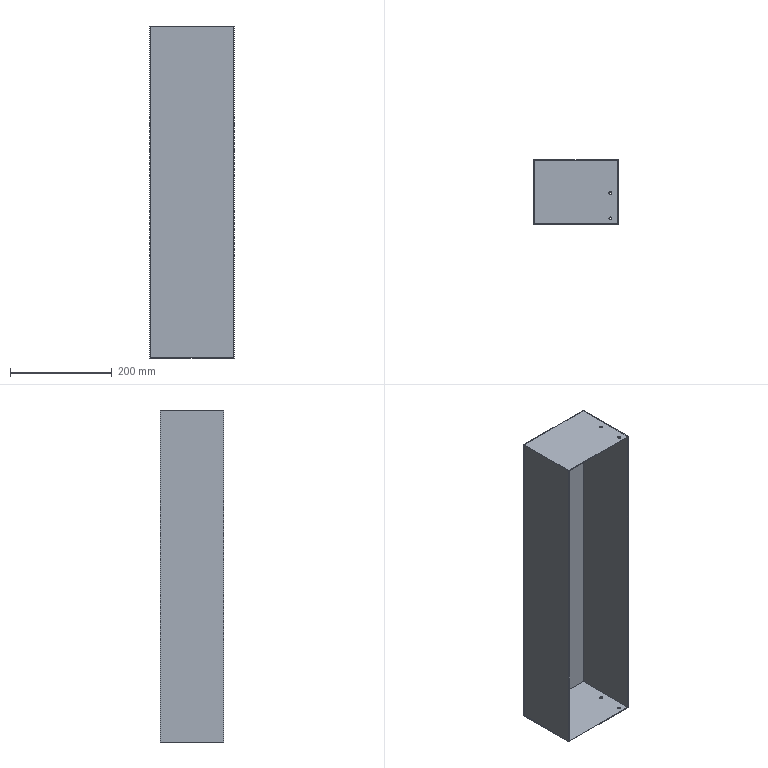Part | STEP file | 1 solid | 19 faces | box 165 x 125 x 652 mm | volume 309587 mm3 | plane 11 | cylinder 8 | commonest cylinder face diameters 6 x8
STEP:
#1=CARTESIAN_POINT('',(0.,0.,0.));
#2=DIRECTION('',(0.,0.,1.));
#3=DIRECTION('',(1.,0.,0.));
#4=AXIS2_PLACEMENT_3D('',#1,#2,#3);
#5=CARTESIAN_POINT('',(-18.,745.,652.));
#6=VERTEX_POINT('',#5);
#7=CARTESIAN_POINT('',(-18.,745.,651.));
#8=VERTEX_POINT('',#7);
#9=CARTESIAN_POINT('',(-18.,745.,652.));
#10=DIRECTION('',(0.,0.,-1.));
#11=VECTOR('',#10,1.);
#12=LINE('',#9,#11);
#13=CARTESIAN_POINT('',(-15.,745.,652.));
#14=DIRECTION('',(0.,0.,-1.));
#15=DIRECTION('',(-1.,0.,0.));
#16=AXIS2_PLACEMENT_3D('',#13,#14,#15);
#17=CYLINDRICAL_SURFACE('',#16,3.);
#18=CARTESIAN_POINT('',(6.283,0.));
#19=DIRECTION('',(0.,1.));
#20=VECTOR('',#19,1.);
#21=LINE('',#18,#20);
#22=(GEOMETRIC_REPRESENTATION_CONTEXT(2)PARAMETRIC_REPRESENTATION_CONTEXT()REPRESENTATION_CONTEXT('',''));
#23=DEFINITIONAL_REPRESENTATION('',(#21),#22);
#24=PCURVE('',#17,#23);
#25=CARTESIAN_POINT('',(-15.,745.,652.));
#26=DIRECTION('',(0.,0.,-1.));
#27=DIRECTION('',(-1.,0.,0.));
#28=AXIS2_PLACEMENT_3D('',#25,#26,#27);
#29=CYLINDRICAL_SURFACE('',#28,3.);
#30=CARTESIAN_POINT('',(0.,0.));
#31=DIRECTION('',(0.,1.));
#32=VECTOR('',#31,1.);
#33=LINE('',#30,#32);
#34=(GEOMETRIC_REPRESENTATION_CONTEXT(2)PARAMETRIC_REPRESENTATION_CONTEXT()REPRESENTATION_CONTEXT('',''));
#35=DEFINITIONAL_REPRESENTATION('',(#33),#34);
#36=PCURVE('',#29,#35);
#37=SURFACE_CURVE('',#12,(#24,#36),.PCURVE_S1.);
#38=EDGE_CURVE('',#6,#8,#37,.T.);
#39=ORIENTED_EDGE('',*,*,#38,.T.);
#40=CARTESIAN_POINT('',(-12.,745.,651.));
#41=VERTEX_POINT('',#40);
#42=CARTESIAN_POINT('',(-15.,745.,651.));
#43=DIRECTION('',(0.,0.,1.));
#44=DIRECTION('',(1.,0.,0.));
#45=AXIS2_PLACEMENT_3D('',#42,#43,#44);
#46=CIRCLE('',#45,3.);
#47=CARTESIAN_POINT('',(9.425,1.));
#48=DIRECTION('',(-1.,0.));
#49=VECTOR('',#48,1.);
#50=LINE('',#47,#49);
#51=(GEOMETRIC_REPRESENTATION_CONTEXT(2)PARAMETRIC_REPRESENTATION_CONTEXT()REPRESENTATION_CONTEXT('',''));
#52=DEFINITIONAL_REPRESENTATION('',(#50),#51);
#53=PCURVE('',#17,#52);
#54=CARTESIAN_POINT('',(0.,0.,651.));
#55=DIRECTION('',(0.,0.,1.));
#56=DIRECTION('',(1.,0.,0.));
#57=AXIS2_PLACEMENT_3D('',#54,#55,#56);
#58=PLANE('',#57);
#59=CARTESIAN_POINT('',(-15.,745.));
#60=DIRECTION('',(1.,0.));
#61=AXIS2_PLACEMENT_2D('',#59,#60);
#62=CIRCLE('',#61,3.);
#63=(GEOMETRIC_REPRESENTATION_CONTEXT(2)PARAMETRIC_REPRESENTATION_CONTEXT()REPRESENTATION_CONTEXT('',''));
#64=DEFINITIONAL_REPRESENTATION('',(#62),#63);
#65=PCURVE('',#58,#64);
#66=SURFACE_CURVE('',#46,(#53,#65),.PCURVE_S1.);
#67=EDGE_CURVE('',#8,#41,#66,.T.);
#68=ORIENTED_EDGE('',*,*,#67,.T.);
#69=CARTESIAN_POINT('',(-12.,745.,652.));
#70=VERTEX_POINT('',#69);
#71=CARTESIAN_POINT('',(-12.,745.,652.));
#72=DIRECTION('',(0.,0.,-1.));
#73=VECTOR('',#72,1.);
#74=LINE('',#71,#73);
#75=CARTESIAN_POINT('',(3.142,0.));
#76=DIRECTION('',(0.,1.));
#77=VECTOR('',#76,1.);
#78=LINE('',#75,#77);
#79=(GEOMETRIC_REPRESENTATION_CONTEXT(2)PARAMETRIC_REPRESENTATION_CONTEXT()REPRESENTATION_CONTEXT('',''));
#80=DEFINITIONAL_REPRESENTATION('',(#78),#79);
#81=PCURVE('',#17,#80);
#82=CARTESIAN_POINT('',(3.142,0.));
#83=DIRECTION('',(0.,1.));
#84=VECTOR('',#83,1.);
#85=LINE('',#82,#84);
#86=(GEOMETRIC_REPRESENTATION_CONTEXT(2)PARAMETRIC_REPRESENTATION_CONTEXT()REPRESENTATION_CONTEXT('',''));
#87=DEFINITIONAL_REPRESENTATION('',(#85),#86);
#88=PCURVE('',#29,#87);
#89=SURFACE_CURVE('',#74,(#81,#88),.PCURVE_S1.);
#90=EDGE_CURVE('',#70,#41,#89,.T.);
#91=ORIENTED_EDGE('',*,*,#90,.F.);
#92=CARTESIAN_POINT('',(-15.,745.,652.));
#93=DIRECTION('',(0.,0.,-1.));
#94=DIRECTION('',(-1.,0.,0.));
#95=AXIS2_PLACEMENT_3D('',#92,#93,#94);
#96=CIRCLE('',#95,3.);
#97=CARTESIAN_POINT('',(0.,0.));
#98=DIRECTION('',(1.,0.));
#99=VECTOR('',#98,1.);
#100=LINE('',#97,#99);
#101=(GEOMETRIC_REPRESENTATION_CONTEXT(2)PARAMETRIC_REPRESENTATION_CONTEXT()REPRESENTATION_CONTEXT('',''));
#102=DEFINITIONAL_REPRESENTATION('',(#100),#101);
#103=PCURVE('',#17,#102);
#104=CARTESIAN_POINT('',(0.,0.,652.));
#105=DIRECTION('',(0.,0.,1.));
#106=DIRECTION('',(1.,0.,0.));
#107=AXIS2_PLACEMENT_3D('',#104,#105,#106);
#108=PLANE('',#107);
#109=CARTESIAN_POINT('',(-18.,745.));
#110=CARTESIAN_POINT('',(-18.,750.196));
#111=CARTESIAN_POINT('',(-13.5,747.598));
#112=CARTESIAN_POINT('',(-9.,745.));
#113=CARTESIAN_POINT('',(-13.5,742.402));
#114=CARTESIAN_POINT('',(-18.,739.804));
#115=CARTESIAN_POINT('',(-18.,745.));
#116=(BOUNDED_CURVE()B_SPLINE_CURVE(2,(#109,#110,#111,#112,#113,#114,#115),.UNSPECIFIED.,.T.,.F.)B_SPLINE_CURVE_WITH_KNOTS((1,2,2,2,2,1),(-2.094,0.,2.094,4.189,6.283,8.378),.UNSPECIFIED.)CURVE()GEOMETRIC_REPRESENTATION_ITEM()RATIONAL_B_SPLINE_CURVE((1.,0.5,1.,0.5,1.,0.5,1.))REPRESENTATION_ITEM(''));
#117=(GEOMETRIC_REPRESENTATION_CONTEXT(2)PARAMETRIC_REPRESENTATION_CONTEXT()REPRESENTATION_CONTEXT('',''));
#118=DEFINITIONAL_REPRESENTATION('',(#116),#117);
#119=PCURVE('',#108,#118);
#120=SURFACE_CURVE('',#96,(#103,#119),.PCURVE_S1.);
#121=EDGE_CURVE('',#70,#6,#120,.T.);
#122=ORIENTED_EDGE('',*,*,#121,.T.);
#123=EDGE_LOOP('',(#39,#68,#91,#122));
#124=FACE_BOUND('',#123,.F.);
#125=ADVANCED_FACE('',(#124),#17,.F.);
#126=CARTESIAN_POINT('',(-18.,745.,1.));
#127=VERTEX_POINT('',#126);
#128=CARTESIAN_POINT('',(-18.,745.,0.));
#129=VERTEX_POINT('',#128);
#130=CARTESIAN_POINT('',(-18.,745.,652.));
#131=DIRECTION('',(0.,0.,-1.));
#132=VECTOR('',#131,1.);
#133=LINE('',#130,#132);
#134=CARTESIAN_POINT('',(-15.,745.,652.));
#135=DIRECTION('',(0.,0.,-1.));
#136=DIRECTION('',(-1.,0.,0.));
#137=AXIS2_PLACEMENT_3D('',#134,#135,#136);
#138=CYLINDRICAL_SURFACE('',#137,3.);
#139=CARTESIAN_POINT('',(6.283,0.));
#140=DIRECTION('',(0.,1.));
#141=VECTOR('',#140,1.);
#142=LINE('',#139,#141);
#143=(GEOMETRIC_REPRESENTATION_CONTEXT(2)PARAMETRIC_REPRESENTATION_CONTEXT()REPRESENTATION_CONTEXT('',''));
#144=DEFINITIONAL_REPRESENTATION('',(#142),#143);
#145=PCURVE('',#138,#144);
#146=CARTESIAN_POINT('',(-15.,745.,652.));
#147=DIRECTION('',(0.,0.,-1.));
#148=DIRECTION('',(-1.,0.,0.));
#149=AXIS2_PLACEMENT_3D('',#146,#147,#148);
#150=CYLINDRICAL_SURFACE('',#149,3.);
#151=CARTESIAN_POINT('',(0.,0.));
#152=DIRECTION('',(0.,1.));
#153=VECTOR('',#152,1.);
#154=LINE('',#151,#153);
#155=(GEOMETRIC_REPRESENTATION_CONTEXT(2)PARAMETRIC_REPRESENTATION_CONTEXT()REPRESENTATION_CONTEXT('',''));
#156=DEFINITIONAL_REPRESENTATION('',(#154),#155);
#157=PCURVE('',#150,#156);
#158=SURFACE_CURVE('',#133,(#145,#157),.PCURVE_S1.);
#159=EDGE_CURVE('',#127,#129,#158,.T.);
#160=ORIENTED_EDGE('',*,*,#159,.T.);
#161=CARTESIAN_POINT('',(-12.,745.,0.));
#162=VERTEX_POINT('',#161);
#163=CARTESIAN_POINT('',(-15.,745.,0.));
#164=DIRECTION('',(0.,0.,-1.));
#165=DIRECTION('',(-1.,0.,0.));
#166=AXIS2_PLACEMENT_3D('',#163,#164,#165);
#167=CIRCLE('',#166,3.);
#168=CARTESIAN_POINT('',(0.,652.));
#169=DIRECTION('',(1.,0.));
#170=VECTOR('',#169,1.);
#171=LINE('',#168,#170);
#172=(GEOMETRIC_REPRESENTATION_CONTEXT(2)PARAMETRIC_REPRESENTATION_CONTEXT()REPRESENTATION_CONTEXT('',''));
#173=DEFINITIONAL_REPRESENTATION('',(#171),#172);
#174=PCURVE('',#138,#173);
#175=CARTESIAN_POINT('',(0.,0.,0.));
#176=DIRECTION('',(0.,0.,1.));
#177=DIRECTION('',(1.,0.,0.));
#178=AXIS2_PLACEMENT_3D('',#175,#176,#177);
#179=PLANE('',#178);
#180=CARTESIAN_POINT('',(-18.,745.));
#181=CARTESIAN_POINT('',(-18.,750.196));
#182=CARTESIAN_POINT('',(-13.5,747.598));
#183=CARTESIAN_POINT('',(-9.,745.));
#184=CARTESIAN_POINT('',(-13.5,742.402));
#185=CARTESIAN_POINT('',(-18.,739.804));
#186=CARTESIAN_POINT('',(-18.,745.));
#187=(BOUNDED_CURVE()B_SPLINE_CURVE(2,(#180,#181,#182,#183,#184,#185,#186),.UNSPECIFIED.,.T.,.F.)B_SPLINE_CURVE_WITH_KNOTS((1,2,2,2,2,1),(-2.094,0.,2.094,4.189,6.283,8.378),.UNSPECIFIED.)CURVE()GEOMETRIC_REPRESENTATION_ITEM()RATIONAL_B_SPLINE_CURVE((1.,0.5,1.,0.5,1.,0.5,1.))REPRESENTATION_ITEM(''));
#188=(GEOMETRIC_REPRESENTATION_CONTEXT(2)PARAMETRIC_REPRESENTATION_CONTEXT()REPRESENTATION_CONTEXT('',''));
#189=DEFINITIONAL_REPRESENTATION('',(#187),#188);
#190=PCURVE('',#179,#189);
#191=SURFACE_CURVE('',#167,(#174,#190),.PCURVE_S1.);
#192=EDGE_CURVE('',#162,#129,#191,.T.);
#193=ORIENTED_EDGE('',*,*,#192,.F.);
#194=CARTESIAN_POINT('',(-12.,745.,1.));
#195=VERTEX_POINT('',#194);
#196=CARTESIAN_POINT('',(-12.,745.,652.));
#197=DIRECTION('',(0.,0.,-1.));
#198=VECTOR('',#197,1.);
#199=LINE('',#196,#198);
#200=CARTESIAN_POINT('',(3.142,0.));
#201=DIRECTION('',(0.,1.));
#202=VECTOR('',#201,1.);
#203=LINE('',#200,#202);
#204=(GEOMETRIC_REPRESENTATION_CONTEXT(2)PARAMETRIC_REPRESENTATION_CONTEXT()REPRESENTATION_CONTEXT('',''));
#205=DEFINITIONAL_REPRESENTATION('',(#203),#204);
#206=PCURVE('',#138,#205);
#207=CARTESIAN_POINT('',(3.142,0.));
#208=DIRECTION('',(0.,1.));
#209=VECTOR('',#208,1.);
#210=LINE('',#207,#209);
#211=(GEOMETRIC_REPRESENTATION_CONTEXT(2)PARAMETRIC_REPRESENTATION_CONTEXT()REPRESENTATION_CONTEXT('',''));
#212=DEFINITIONAL_REPRESENTATION('',(#210),#211);
#213=PCURVE('',#150,#212);
#214=SURFACE_CURVE('',#199,(#206,#213),.PCURVE_S1.);
#215=EDGE_CURVE('',#195,#162,#214,.T.);
#216=ORIENTED_EDGE('',*,*,#215,.F.);
#217=CARTESIAN_POINT('',(-15.,745.,1.));
#218=DIRECTION('',(0.,0.,1.));
#219=DIRECTION('',(1.,0.,0.));
#220=AXIS2_PLACEMENT_3D('',#217,#218,#219);
#221=CIRCLE('',#220,3.);
#222=CARTESIAN_POINT('',(9.425,651.));
#223=DIRECTION('',(-1.,0.));
#224=VECTOR('',#223,1.);
#225=LINE('',#222,#224);
#226=(GEOMETRIC_REPRESENTATION_CONTEXT(2)PARAMETRIC_REPRESENTATION_CONTEXT()REPRESENTATION_CONTEXT('',''));
#227=DEFINITIONAL_REPRESENTATION('',(#225),#226);
#228=PCURVE('',#138,#227);
#229=CARTESIAN_POINT('',(0.,0.,1.));
#230=DIRECTION('',(0.,0.,1.));
#231=DIRECTION('',(1.,0.,0.));
#232=AXIS2_PLACEMENT_3D('',#229,#230,#231);
#233=PLANE('',#232);
#234=CARTESIAN_POINT('',(-15.,745.));
#235=DIRECTION('',(1.,0.));
#236=AXIS2_PLACEMENT_2D('',#234,#235);
#237=CIRCLE('',#236,3.);
#238=(GEOMETRIC_REPRESENTATION_CONTEXT(2)PARAMETRIC_REPRESENTATION_CONTEXT()REPRESENTATION_CONTEXT('',''));
#239=DEFINITIONAL_REPRESENTATION('',(#237),#238);
#240=PCURVE('',#233,#239);
#241=SURFACE_CURVE('',#221,(#228,#240),.PCURVE_S1.);
#242=EDGE_CURVE('',#127,#195,#241,.T.);
#243=ORIENTED_EDGE('',*,*,#242,.F.);
#244=EDGE_LOOP('',(#160,#193,#216,#243));
#245=FACE_BOUND('',#244,.F.);
#246=ADVANCED_FACE('',(#245),#138,.F.);
#247=CARTESIAN_POINT('',(-18.,695.,652.));
#248=VERTEX_POINT('',#247);
#249=CARTESIAN_POINT('',(-18.,695.,651.));
#250=VERTEX_POINT('',#249);
#251=CARTESIAN_POINT('',(-18.,695.,652.));
#252=DIRECTION('',(0.,0.,-1.));
#253=VECTOR('',#252,1.);
#254=LINE('',#251,#253);
#255=CARTESIAN_POINT('',(-15.,695.,652.));
#256=DIRECTION('',(0.,0.,-1.));
#257=DIRECTION('',(-1.,0.,0.));
#258=AXIS2_PLACEMENT_3D('',#255,#256,#257);
#259=CYLINDRICAL_SURFACE('',#258,3.);
#260=CARTESIAN_POINT('',(6.283,0.));
#261=DIRECTION('',(0.,1.));
#262=VECTOR('',#261,1.);
#263=LINE('',#260,#262);
#264=(GEOMETRIC_REPRESENTATION_CONTEXT(2)PARAMETRIC_REPRESENTATION_CONTEXT()REPRESENTATION_CONTEXT('',''));
#265=DEFINITIONAL_REPRESENTATION('',(#263),#264);
#266=PCURVE('',#259,#265);
#267=CARTESIAN_POINT('',(-15.,695.,652.));
#268=DIRECTION('',(0.,0.,-1.));
#269=DIRECTION('',(-1.,0.,0.));
#270=AXIS2_PLACEMENT_3D('',#267,#268,#269);
#271=CYLINDRICAL_SURFACE('',#270,3.);
#272=CARTESIAN_POINT('',(0.,0.));
#273=DIRECTION('',(0.,1.));
#274=VECTOR('',#273,1.);
#275=LINE('',#272,#274);
#276=(GEOMETRIC_REPRESENTATION_CONTEXT(2)PARAMETRIC_REPRESENTATION_CONTEXT()REPRESENTATION_CONTEXT('',''));
#277=DEFINITIONAL_REPRESENTATION('',(#275),#276);
#278=PCURVE('',#271,#277);
#279=SURFACE_CURVE('',#254,(#266,#278),.PCURVE_S1.);
#280=EDGE_CURVE('',#248,#250,#279,.T.);
#281=ORIENTED_EDGE('',*,*,#280,.T.);
#282=CARTESIAN_POINT('',(-12.,695.,651.));
#283=VERTEX_POINT('',#282);
#284=CARTESIAN_POINT('',(-15.,695.,651.));
#285=DIRECTION('',(0.,0.,1.));
#286=DIRECTION('',(1.,0.,0.));
#287=AXIS2_PLACEMENT_3D('',#284,#285,#286);
#288=CIRCLE('',#287,3.);
#289=CARTESIAN_POINT('',(9.425,1.));
#290=DIRECTION('',(-1.,0.));
#291=VECTOR('',#290,1.);
#292=LINE('',#289,#291);
#293=(GEOMETRIC_REPRESENTATION_CONTEXT(2)PARAMETRIC_REPRESENTATION_CONTEXT()REPRESENTATION_CONTEXT('',''));
#294=DEFINITIONAL_REPRESENTATION('',(#292),#293);
#295=PCURVE('',#259,#294);
#296=CARTESIAN_POINT('',(-15.,695.));
#297=DIRECTION('',(1.,0.));
#298=AXIS2_PLACEMENT_2D('',#296,#297);
#299=CIRCLE('',#298,3.);
#300=(GEOMETRIC_REPRESENTATION_CONTEXT(2)PARAMETRIC_REPRESENTATION_CONTEXT()REPRESENTATION_CONTEXT('',''));
#301=DEFINITIONAL_REPRESENTATION('',(#299),#300);
#302=PCURVE('',#58,#301);
#303=SURFACE_CURVE('',#288,(#295,#302),.PCURVE_S1.);
#304=EDGE_CURVE('',#250,#283,#303,.T.);
#305=ORIENTED_EDGE('',*,*,#304,.T.);
#306=CARTESIAN_POINT('',(-12.,695.,652.));
#307=VERTEX_POINT('',#306);
#308=CARTESIAN_POINT('',(-12.,695.,652.));
#309=DIRECTION('',(0.,0.,-1.));
#310=VECTOR('',#309,1.);
#311=LINE('',#308,#310);
#312=CARTESIAN_POINT('',(3.142,0.));
#313=DIRECTION('',(0.,1.));
#314=VECTOR('',#313,1.);
#315=LINE('',#312,#314);
#316=(GEOMETRIC_REPRESENTATION_CONTEXT(2)PARAMETRIC_REPRESENTATION_CONTEXT()REPRESENTATION_CONTEXT('',''));
#317=DEFINITIONAL_REPRESENTATION('',(#315),#316);
#318=PCURVE('',#259,#317);
#319=CARTESIAN_POINT('',(3.142,0.));
#320=DIRECTION('',(0.,1.));
#321=VECTOR('',#320,1.);
#322=LINE('',#319,#321);
#323=(GEOMETRIC_REPRESENTATION_CONTEXT(2)PARAMETRIC_REPRESENTATION_CONTEXT()REPRESENTATION_CONTEXT('',''));
#324=DEFINITIONAL_REPRESENTATION('',(#322),#323);
#325=PCURVE('',#271,#324);
#326=SURFACE_CURVE('',#311,(#318,#325),.PCURVE_S1.);
#327=EDGE_CURVE('',#307,#283,#326,.T.);
#328=ORIENTED_EDGE('',*,*,#327,.F.);
#329=CARTESIAN_POINT('',(-15.,695.,652.));
#330=DIRECTION('',(0.,0.,-1.));
#331=DIRECTION('',(-1.,0.,0.));
#332=AXIS2_PLACEMENT_3D('',#329,#330,#331);
#333=CIRCLE('',#332,3.);
#334=CARTESIAN_POINT('',(0.,0.));
#335=DIRECTION('',(1.,0.));
#336=VECTOR('',#335,1.);
#337=LINE('',#334,#336);
#338=(GEOMETRIC_REPRESENTATION_CONTEXT(2)PARAMETRIC_REPRESENTATION_CONTEXT()REPRESENTATION_CONTEXT('',''));
#339=DEFINITIONAL_REPRESENTATION('',(#337),#338);
#340=PCURVE('',#259,#339);
#341=CARTESIAN_POINT('',(-18.,695.));
#342=CARTESIAN_POINT('',(-18.,700.196));
#343=CARTESIAN_POINT('',(-13.5,697.598));
#344=CARTESIAN_POINT('',(-9.,695.));
#345=CARTESIAN_POINT('',(-13.5,692.402));
#346=CARTESIAN_POINT('',(-18.,689.804));
#347=CARTESIAN_POINT('',(-18.,695.));
#348=(BOUNDED_CURVE()B_SPLINE_CURVE(2,(#341,#342,#343,#344,#345,#346,#347),.UNSPECIFIED.,.T.,.F.)B_SPLINE_CURVE_WITH_KNOTS((1,2,2,2,2,1),(-2.094,0.,2.094,4.189,6.283,8.378),.UNSPECIFIED.)CURVE()GEOMETRIC_REPRESENTATION_ITEM()RATIONAL_B_SPLINE_CURVE((1.,0.5,1.,0.5,1.,0.5,1.))REPRESENTATION_ITEM(''));
#349=(GEOMETRIC_REPRESENTATION_CONTEXT(2)PARAMETRIC_REPRESENTATION_CONTEXT()REPRESENTATION_CONTEXT('',''));
#350=DEFINITIONAL_REPRESENTATION('',(#348),#349);
#351=PCURVE('',#108,#350);
#352=SURFACE_CURVE('',#333,(#340,#351),.PCURVE_S1.);
#353=EDGE_CURVE('',#307,#248,#352,.T.);
#354=ORIENTED_EDGE('',*,*,#353,.T.);
#355=EDGE_LOOP('',(#281,#305,#328,#354));
#356=FACE_BOUND('',#355,.F.);
#357=ADVANCED_FACE('',(#356),#259,.F.);
#358=CARTESIAN_POINT('',(-18.,695.,1.));
#359=VERTEX_POINT('',#358);
#360=CARTESIAN_POINT('',(-18.,695.,0.));
#361=VERTEX_POINT('',#360);
#362=CARTESIAN_POINT('',(-18.,695.,652.));
#363=DIRECTION('',(0.,0.,-1.));
#364=VECTOR('',#363,1.);
#365=LINE('',#362,#364);
#366=CARTESIAN_POINT('',(-15.,695.,652.));
#367=DIRECTION('',(0.,0.,-1.));
#368=DIRECTION('',(-1.,0.,0.));
#369=AXIS2_PLACEMENT_3D('',#366,#367,#368);
#370=CYLINDRICAL_SURFACE('',#369,3.);
#371=CARTESIAN_POINT('',(6.283,0.));
#372=DIRECTION('',(0.,1.));
#373=VECTOR('',#372,1.);
#374=LINE('',#371,#373);
#375=(GEOMETRIC_REPRESENTATION_CONTEXT(2)PARAMETRIC_REPRESENTATION_CONTEXT()REPRESENTATION_CONTEXT('',''));
#376=DEFINITIONAL_REPRESENTATION('',(#374),#375);
#377=PCURVE('',#370,#376);
#378=CARTESIAN_POINT('',(-15.,695.,652.));
#379=DIRECTION('',(0.,0.,-1.));
#380=DIRECTION('',(-1.,0.,0.));
#381=AXIS2_PLACEMENT_3D('',#378,#379,#380);
#382=CYLINDRICAL_SURFACE('',#381,3.);
#383=CARTESIAN_POINT('',(0.,0.));
#384=DIRECTION('',(0.,1.));
#385=VECTOR('',#384,1.);
#386=LINE('',#383,#385);
#387=(GEOMETRIC_REPRESENTATION_CONTEXT(2)PARAMETRIC_REPRESENTATION_CONTEXT()REPRESENTATION_CONTEXT('',''));
#388=DEFINITIONAL_REPRESENTATION('',(#386),#387);
#389=PCURVE('',#382,#388);
#390=SURFACE_CURVE('',#365,(#377,#389),.PCURVE_S1.);
#391=EDGE_CURVE('',#359,#361,#390,.T.);
#392=ORIENTED_EDGE('',*,*,#391,.T.);
#393=CARTESIAN_POINT('',(-12.,695.,0.));
#394=VERTEX_POINT('',#393);
#395=CARTESIAN_POINT('',(-15.,695.,0.));
#396=DIRECTION('',(0.,0.,-1.));
#397=DIRECTION('',(-1.,0.,0.));
#398=AXIS2_PLACEMENT_3D('',#395,#396,#397);
#399=CIRCLE('',#398,3.);
#400=CARTESIAN_POINT('',(0.,652.));
#401=DIRECTION('',(1.,0.));
#402=VECTOR('',#401,1.);
#403=LINE('',#400,#402);
#404=(GEOMETRIC_REPRESENTATION_CONTEXT(2)PARAMETRIC_REPRESENTATION_CONTEXT()REPRESENTATION_CONTEXT('',''));
#405=DEFINITIONAL_REPRESENTATION('',(#403),#404);
#406=PCURVE('',#370,#405);
#407=CARTESIAN_POINT('',(-18.,695.));
#408=CARTESIAN_POINT('',(-18.,700.196));
#409=CARTESIAN_POINT('',(-13.5,697.598));
#410=CARTESIAN_POINT('',(-9.,695.));
#411=CARTESIAN_POINT('',(-13.5,692.402));
#412=CARTESIAN_POINT('',(-18.,689.804));
#413=CARTESIAN_POINT('',(-18.,695.));
#414=(BOUNDED_CURVE()B_SPLINE_CURVE(2,(#407,#408,#409,#410,#411,#412,#413),.UNSPECIFIED.,.T.,.F.)B_SPLINE_CURVE_WITH_KNOTS((1,2,2,2,2,1),(-2.094,0.,2.094,4.189,6.283,8.378),.UNSPECIFIED.)CURVE()GEOMETRIC_REPRESENTATION_ITEM()RATIONAL_B_SPLINE_CURVE((1.,0.5,1.,0.5,1.,0.5,1.))REPRESENTATION_ITEM(''));
#415=(GEOMETRIC_REPRESENTATION_CONTEXT(2)PARAMETRIC_REPRESENTATION_CONTEXT()REPRESENTATION_CONTEXT('',''));
#416=DEFINITIONAL_REPRESENTATION('',(#414),#415);
#417=PCURVE('',#179,#416);
#418=SURFACE_CURVE('',#399,(#406,#417),.PCURVE_S1.);
#419=EDGE_CURVE('',#394,#361,#418,.T.);
#420=ORIENTED_EDGE('',*,*,#419,.F.);
#421=CARTESIAN_POINT('',(-12.,695.,1.));
#422=VERTEX_POINT('',#421);
#423=CARTESIAN_POINT('',(-12.,695.,652.));
#424=DIRECTION('',(0.,0.,-1.));
#425=VECTOR('',#424,1.);
#426=LINE('',#423,#425);
#427=CARTESIAN_POINT('',(3.142,0.));
#428=DIRECTION('',(0.,1.));
#429=VECTOR('',#428,1.);
#430=LINE('',#427,#429);
#431=(GEOMETRIC_REPRESENTATION_CONTEXT(2)PARAMETRIC_REPRESENTATION_CONTEXT()REPRESENTATION_CONTEXT('',''));
#432=DEFINITIONAL_REPRESENTATION('',(#430),#431);
#433=PCURVE('',#370,#432);
#434=CARTESIAN_POINT('',(3.142,0.));
#435=DIRECTION('',(0.,1.));
#436=VECTOR('',#435,1.);
#437=LINE('',#434,#436);
#438=(GEOMETRIC_REPRESENTATION_CONTEXT(2)PARAMETRIC_REPRESENTATION_CONTEXT()REPRESENTATION_CONTEXT('',''));
#439=DEFINITIONAL_REPRESENTATION('',(#437),#438);
#440=PCURVE('',#382,#439);
#441=SURFACE_CURVE('',#426,(#433,#440),.PCURVE_S1.);
#442=EDGE_CURVE('',#422,#394,#441,.T.);
#443=ORIENTED_EDGE('',*,*,#442,.F.);
#444=CARTESIAN_POINT('',(-15.,695.,1.));
#445=DIRECTION('',(0.,0.,1.));
#446=DIRECTION('',(1.,0.,0.));
#447=AXIS2_PLACEMENT_3D('',#444,#445,#446);
#448=CIRCLE('',#447,3.);
#449=CARTESIAN_POINT('',(9.425,651.));
#450=DIRECTION('',(-1.,0.));
#451=VECTOR('',#450,1.);
#452=LINE('',#449,#451);
#453=(GEOMETRIC_REPRESENTATION_CONTEXT(2)PARAMETRIC_REPRESENTATION_CONTEXT()REPRESENTATION_CONTEXT('',''));
#454=DEFINITIONAL_REPRESENTATION('',(#452),#453);
#455=PCURVE('',#370,#454);
#456=CARTESIAN_POINT('',(-15.,695.));
#457=DIRECTION('',(1.,0.));
#458=AXIS2_PLACEMENT_2D('',#456,#457);
#459=CIRCLE('',#458,3.);
#460=(GEOMETRIC_REPRESENTATION_CONTEXT(2)PARAMETRIC_REPRESENTATION_CONTEXT()REPRESENTATION_CONTEXT('',''));
#461=DEFINITIONAL_REPRESENTATION('',(#459),#460);
#462=PCURVE('',#233,#461);
#463=SURFACE_CURVE('',#448,(#455,#462),.PCURVE_S1.);
#464=EDGE_CURVE('',#359,#422,#463,.T.);
#465=ORIENTED_EDGE('',*,*,#464,.F.);
#466=EDGE_LOOP('',(#392,#420,#443,#465));
#467=FACE_BOUND('',#466,.F.);
#468=ADVANCED_FACE('',(#467),#370,.F.);
#469=CARTESIAN_POINT('',(0.,810.,0.));
#470=VERTEX_POINT('',#469);
#471=CARTESIAN_POINT('',(-165.,810.,0.));
#472=VERTEX_POINT('',#471);
#473=CARTESIAN_POINT('',(0.,810.,0.));
#474=DIRECTION('',(-1.,0.,0.));
#475=VECTOR('',#474,1.);
#476=LINE('',#473,#475);
#477=CARTESIAN_POINT('',(0.,810.,652.));
#478=DIRECTION('',(0.,-1.,0.));
#479=DIRECTION('',(1.,0.,0.));
#480=AXIS2_PLACEMENT_3D('',#477,#478,#479);
#481=PLANE('',#480);
#482=CARTESIAN_POINT('',(0.,-652.));
#483=DIRECTION('',(-1.,0.));
#484=VECTOR('',#483,1.);
#485=LINE('',#482,#484);
#486=(GEOMETRIC_REPRESENTATION_CONTEXT(2)PARAMETRIC_REPRESENTATION_CONTEXT()REPRESENTATION_CONTEXT('',''));
#487=DEFINITIONAL_REPRESENTATION('',(#485),#486);
#488=PCURVE('',#481,#487);
#489=CARTESIAN_POINT('',(0.,810.));
#490=DIRECTION('',(-1.,0.));
#491=VECTOR('',#490,1.);
#492=LINE('',#489,#491);
#493=(GEOMETRIC_REPRESENTATION_CONTEXT(2)PARAMETRIC_REPRESENTATION_CONTEXT()REPRESENTATION_CONTEXT('',''));
#494=DEFINITIONAL_REPRESENTATION('',(#492),#493);
#495=PCURVE('',#179,#494);
#496=SURFACE_CURVE('',#476,(#488,#495),.PCURVE_S1.);
#497=EDGE_CURVE('',#470,#472,#496,.T.);
#498=ORIENTED_EDGE('',*,*,#497,.T.);
#499=CARTESIAN_POINT('',(-165.,810.,652.));
#500=VERTEX_POINT('',#499);
#501=CARTESIAN_POINT('',(-165.,810.,652.));
#502=DIRECTION('',(0.,0.,-1.));
#503=VECTOR('',#502,1.);
#504=LINE('',#501,#503);
#505=CARTESIAN_POINT('',(-165.,0.));
#506=DIRECTION('',(0.,-1.));
#507=VECTOR('',#506,1.);
#508=LINE('',#505,#507);
#509=(GEOMETRIC_REPRESENTATION_CONTEXT(2)PARAMETRIC_REPRESENTATION_CONTEXT()REPRESENTATION_CONTEXT('',''));
#510=DEFINITIONAL_REPRESENTATION('',(#508),#509);
#511=PCURVE('',#481,#510);
#512=CARTESIAN_POINT('',(-165.,0.,652.));
#513=DIRECTION('',(1.,0.,0.));
#514=DIRECTION('',(0.,0.,-1.));
#515=AXIS2_PLACEMENT_3D('',#512,#513,#514);
#516=PLANE('',#515);
#517=CARTESIAN_POINT('',(0.,810.));
#518=DIRECTION('',(1.,0.));
#519=VECTOR('',#518,1.);
#520=LINE('',#517,#519);
#521=(GEOMETRIC_REPRESENTATION_CONTEXT(2)PARAMETRIC_REPRESENTATION_CONTEXT()REPRESENTATION_CONTEXT('',''));
#522=DEFINITIONAL_REPRESENTATION('',(#520),#521);
#523=PCURVE('',#516,#522);
#524=SURFACE_CURVE('',#504,(#511,#523),.PCURVE_S1.);
#525=EDGE_CURVE('',#500,#472,#524,.T.);
#526=ORIENTED_EDGE('',*,*,#525,.F.);
#527=CARTESIAN_POINT('',(0.,810.,652.));
#528=VERTEX_POINT('',#527);
#529=CARTESIAN_POINT('',(0.,810.,652.));
#530=DIRECTION('',(-1.,0.,0.));
#531=VECTOR('',#530,1.);
#532=LINE('',#529,#531);
#533=CARTESIAN_POINT('',(0.,0.));
#534=DIRECTION('',(-1.,0.));
#535=VECTOR('',#534,1.);
#536=LINE('',#533,#535);
#537=(GEOMETRIC_REPRESENTATION_CONTEXT(2)PARAMETRIC_REPRESENTATION_CONTEXT()REPRESENTATION_CONTEXT('',''));
#538=DEFINITIONAL_REPRESENTATION('',(#536),#537);
#539=PCURVE('',#481,#538);
#540=CARTESIAN_POINT('',(0.,810.));
#541=DIRECTION('',(-1.,0.));
#542=VECTOR('',#541,1.);
#543=LINE('',#540,#542);
#544=(GEOMETRIC_REPRESENTATION_CONTEXT(2)PARAMETRIC_REPRESENTATION_CONTEXT()REPRESENTATION_CONTEXT('',''));
#545=DEFINITIONAL_REPRESENTATION('',(#543),#544);
#546=PCURVE('',#108,#545);
#547=SURFACE_CURVE('',#532,(#539,#546),.PCURVE_S1.);
#548=EDGE_CURVE('',#528,#500,#547,.T.);
#549=ORIENTED_EDGE('',*,*,#548,.F.);
#550=CARTESIAN_POINT('',(0.,810.,652.));
#551=DIRECTION('',(0.,0.,-1.));
#552=VECTOR('',#551,1.);
#553=LINE('',#550,#552);
#554=CARTESIAN_POINT('',(0.,0.));
#555=DIRECTION('',(0.,-1.));
#556=VECTOR('',#555,1.);
#557=LINE('',#554,#556);
#558=(GEOMETRIC_REPRESENTATION_CONTEXT(2)PARAMETRIC_REPRESENTATION_CONTEXT()REPRESENTATION_CONTEXT('',''));
#559=DEFINITIONAL_REPRESENTATION('',(#557),#558);
#560=PCURVE('',#481,#559);
#561=CARTESIAN_POINT('',(0.,0.,652.));
#562=DIRECTION('',(-1.,0.,0.));
#563=DIRECTION('',(0.,0.,1.));
#564=AXIS2_PLACEMENT_3D('',#561,#562,#563);
#565=PLANE('',#564);
#566=CARTESIAN_POINT('',(0.,810.));
#567=DIRECTION('',(-1.,0.));
#568=VECTOR('',#567,1.);
#569=LINE('',#566,#568);
#570=(GEOMETRIC_REPRESENTATION_CONTEXT(2)PARAMETRIC_REPRESENTATION_CONTEXT()REPRESENTATION_CONTEXT('',''));
#571=DEFINITIONAL_REPRESENTATION('',(#569),#570);
#572=PCURVE('',#565,#571);
#573=SURFACE_CURVE('',#553,(#560,#572),.PCURVE_S1.);
#574=EDGE_CURVE('',#528,#470,#573,.T.);
#575=ORIENTED_EDGE('',*,*,#574,.T.);
#576=EDGE_LOOP('',(#498,#526,#549,#575));
#577=FACE_BOUND('',#576,.T.);
#578=ADVANCED_FACE('',(#577),#481,.F.);
#579=CARTESIAN_POINT('',(-165.,685.,0.));
#580=VERTEX_POINT('',#579);
#581=CARTESIAN_POINT('',(-165.,0.,0.));
#582=DIRECTION('',(0.,-1.,0.));
#583=VECTOR('',#582,1.);
#584=LINE('',#581,#583);
#585=CARTESIAN_POINT('',(652.,0.));
#586=DIRECTION('',(0.,-1.));
#587=VECTOR('',#586,1.);
#588=LINE('',#585,#587);
#589=(GEOMETRIC_REPRESENTATION_CONTEXT(2)PARAMETRIC_REPRESENTATION_CONTEXT()REPRESENTATION_CONTEXT('',''));
#590=DEFINITIONAL_REPRESENTATION('',(#588),#589);
#591=PCURVE('',#516,#590);
#592=CARTESIAN_POINT('',(-165.,0.));
#593=DIRECTION('',(0.,-1.));
#594=VECTOR('',#593,1.);
#595=LINE('',#592,#594);
#596=(GEOMETRIC_REPRESENTATION_CONTEXT(2)PARAMETRIC_REPRESENTATION_CONTEXT()REPRESENTATION_CONTEXT('',''));
#597=DEFINITIONAL_REPRESENTATION('',(#595),#596);
#598=PCURVE('',#179,#597);
#599=SURFACE_CURVE('',#584,(#591,#598),.PCURVE_S1.);
#600=EDGE_CURVE('',#472,#580,#599,.T.);
#601=ORIENTED_EDGE('',*,*,#600,.T.);
#602=CARTESIAN_POINT('',(-165.,685.,652.));
#603=VERTEX_POINT('',#602);
#604=CARTESIAN_POINT('',(-165.,685.,652.));
#605=DIRECTION('',(0.,0.,-1.));
#606=VECTOR('',#605,1.);
#607=LINE('',#604,#606);
#608=CARTESIAN_POINT('',(0.,685.));
#609=DIRECTION('',(1.,0.));
#610=VECTOR('',#609,1.);
#611=LINE('',#608,#610);
#612=(GEOMETRIC_REPRESENTATION_CONTEXT(2)PARAMETRIC_REPRESENTATION_CONTEXT()REPRESENTATION_CONTEXT('',''));
#613=DEFINITIONAL_REPRESENTATION('',(#611),#612);
#614=PCURVE('',#516,#613);
#615=CARTESIAN_POINT('',(0.,685.,652.));
#616=DIRECTION('',(0.,1.,0.));
#617=DIRECTION('',(-1.,0.,0.));
#618=AXIS2_PLACEMENT_3D('',#615,#616,#617);
#619=PLANE('',#618);
#620=CARTESIAN_POINT('',(165.,0.));
#621=DIRECTION('',(0.,-1.));
#622=VECTOR('',#621,1.);
#623=LINE('',#620,#622);
#624=(GEOMETRIC_REPRESENTATION_CONTEXT(2)PARAMETRIC_REPRESENTATION_CONTEXT()REPRESENTATION_CONTEXT('',''));
#625=DEFINITIONAL_REPRESENTATION('',(#623),#624);
#626=PCURVE('',#619,#625);
#627=SURFACE_CURVE('',#607,(#614,#626),.PCURVE_S1.);
#628=EDGE_CURVE('',#603,#580,#627,.T.);
#629=ORIENTED_EDGE('',*,*,#628,.F.);
#630=CARTESIAN_POINT('',(-165.,0.,652.));
#631=DIRECTION('',(0.,-1.,0.));
#632=VECTOR('',#631,1.);
#633=LINE('',#630,#632);
#634=CARTESIAN_POINT('',(0.,0.));
#635=DIRECTION('',(0.,-1.));
#636=VECTOR('',#635,1.);
#637=LINE('',#634,#636);
#638=(GEOMETRIC_REPRESENTATION_CONTEXT(2)PARAMETRIC_REPRESENTATION_CONTEXT()REPRESENTATION_CONTEXT('',''));
#639=DEFINITIONAL_REPRESENTATION('',(#637),#638);
#640=PCURVE('',#516,#639);
#641=CARTESIAN_POINT('',(-165.,0.));
#642=DIRECTION('',(0.,-1.));
#643=VECTOR('',#642,1.);
#644=LINE('',#641,#643);
#645=(GEOMETRIC_REPRESENTATION_CONTEXT(2)PARAMETRIC_REPRESENTATION_CONTEXT()REPRESENTATION_CONTEXT('',''));
#646=DEFINITIONAL_REPRESENTATION('',(#644),#645);
#647=PCURVE('',#108,#646);
#648=SURFACE_CURVE('',#633,(#640,#647),.PCURVE_S1.);
#649=EDGE_CURVE('',#500,#603,#648,.T.);
#650=ORIENTED_EDGE('',*,*,#649,.F.);
#651=ORIENTED_EDGE('',*,*,#525,.T.);
#652=EDGE_LOOP('',(#601,#629,#650,#651));
#653=FACE_BOUND('',#652,.T.);
#654=ADVANCED_FACE('',(#653),#516,.F.);
#655=CARTESIAN_POINT('',(0.,685.,652.));
#656=VERTEX_POINT('',#655);
#657=CARTESIAN_POINT('',(0.,0.,652.));
#658=DIRECTION('',(0.,1.,0.));
#659=VECTOR('',#658,1.);
#660=LINE('',#657,#659);
#661=CARTESIAN_POINT('',(0.,0.));
#662=DIRECTION('',(0.,1.));
#663=VECTOR('',#662,1.);
#664=LINE('',#661,#663);
#665=(GEOMETRIC_REPRESENTATION_CONTEXT(2)PARAMETRIC_REPRESENTATION_CONTEXT()REPRESENTATION_CONTEXT('',''));
#666=DEFINITIONAL_REPRESENTATION('',(#664),#665);
#667=PCURVE('',#565,#666);
#668=CARTESIAN_POINT('',(0.,0.));
#669=DIRECTION('',(0.,1.));
#670=VECTOR('',#669,1.);
#671=LINE('',#668,#670);
#672=(GEOMETRIC_REPRESENTATION_CONTEXT(2)PARAMETRIC_REPRESENTATION_CONTEXT()REPRESENTATION_CONTEXT('',''));
#673=DEFINITIONAL_REPRESENTATION('',(#671),#672);
#674=PCURVE('',#108,#673);
#675=SURFACE_CURVE('',#660,(#667,#674),.PCURVE_S1.);
#676=EDGE_CURVE('',#656,#528,#675,.T.);
#677=ORIENTED_EDGE('',*,*,#676,.F.);
#678=CARTESIAN_POINT('',(0.,685.,0.));
#679=VERTEX_POINT('',#678);
#680=CARTESIAN_POINT('',(0.,685.,652.));
#681=DIRECTION('',(0.,0.,-1.));
#682=VECTOR('',#681,1.);
#683=LINE('',#680,#682);
#684=CARTESIAN_POINT('',(0.,685.));
#685=DIRECTION('',(-1.,0.));
#686=VECTOR('',#685,1.);
#687=LINE('',#684,#686);
#688=(GEOMETRIC_REPRESENTATION_CONTEXT(2)PARAMETRIC_REPRESENTATION_CONTEXT()REPRESENTATION_CONTEXT('',''));
#689=DEFINITIONAL_REPRESENTATION('',(#687),#688);
#690=PCURVE('',#565,#689);
#691=CARTESIAN_POINT('',(0.,0.));
#692=DIRECTION('',(0.,-1.));
#693=VECTOR('',#692,1.);
#694=LINE('',#691,#693);
#695=(GEOMETRIC_REPRESENTATION_CONTEXT(2)PARAMETRIC_REPRESENTATION_CONTEXT()REPRESENTATION_CONTEXT('',''));
#696=DEFINITIONAL_REPRESENTATION('',(#694),#695);
#697=PCURVE('',#619,#696);
#698=SURFACE_CURVE('',#683,(#690,#697),.PCURVE_S1.);
#699=EDGE_CURVE('',#656,#679,#698,.T.);
#700=ORIENTED_EDGE('',*,*,#699,.T.);
#701=CARTESIAN_POINT('',(0.,0.,0.));
#702=DIRECTION('',(0.,1.,0.));
#703=VECTOR('',#702,1.);
#704=LINE('',#701,#703);
#705=CARTESIAN_POINT('',(-652.,0.));
#706=DIRECTION('',(0.,1.));
#707=VECTOR('',#706,1.);
#708=LINE('',#705,#707);
#709=(GEOMETRIC_REPRESENTATION_CONTEXT(2)PARAMETRIC_REPRESENTATION_CONTEXT()REPRESENTATION_CONTEXT('',''));
#710=DEFINITIONAL_REPRESENTATION('',(#708),#709);
#711=PCURVE('',#565,#710);
#712=CARTESIAN_POINT('',(0.,0.));
#713=DIRECTION('',(0.,1.));
#714=VECTOR('',#713,1.);
#715=LINE('',#712,#714);
#716=(GEOMETRIC_REPRESENTATION_CONTEXT(2)PARAMETRIC_REPRESENTATION_CONTEXT()REPRESENTATION_CONTEXT('',''));
#717=DEFINITIONAL_REPRESENTATION('',(#715),#716);
#718=PCURVE('',#179,#717);
#719=SURFACE_CURVE('',#704,(#711,#718),.PCURVE_S1.);
#720=EDGE_CURVE('',#679,#470,#719,.T.);
#721=ORIENTED_EDGE('',*,*,#720,.T.);
#722=ORIENTED_EDGE('',*,*,#574,.F.);
#723=EDGE_LOOP('',(#677,#700,#721,#722));
#724=FACE_BOUND('',#723,.T.);
#725=ADVANCED_FACE('',(#724),#565,.F.);
#726=CARTESIAN_POINT('',(-15.,745.,652.));
#727=DIRECTION('',(0.,0.,-1.));
#728=DIRECTION('',(-1.,0.,0.));
#729=AXIS2_PLACEMENT_3D('',#726,#727,#728);
#730=CIRCLE('',#729,3.);
#731=CARTESIAN_POINT('',(-18.,745.));
#732=CARTESIAN_POINT('',(-18.,750.196));
#733=CARTESIAN_POINT('',(-13.5,747.598));
#734=CARTESIAN_POINT('',(-9.,745.));
#735=CARTESIAN_POINT('',(-13.5,742.402));
#736=CARTESIAN_POINT('',(-18.,739.804));
#737=CARTESIAN_POINT('',(-18.,745.));
#738=(BOUNDED_CURVE()B_SPLINE_CURVE(2,(#731,#732,#733,#734,#735,#736,#737),.UNSPECIFIED.,.T.,.F.)B_SPLINE_CURVE_WITH_KNOTS((1,2,2,2,2,1),(-2.094,0.,2.094,4.189,6.283,8.378),.UNSPECIFIED.)CURVE()GEOMETRIC_REPRESENTATION_ITEM()RATIONAL_B_SPLINE_CURVE((1.,0.5,1.,0.5,1.,0.5,1.))REPRESENTATION_ITEM(''));
#739=(GEOMETRIC_REPRESENTATION_CONTEXT(2)PARAMETRIC_REPRESENTATION_CONTEXT()REPRESENTATION_CONTEXT('',''));
#740=DEFINITIONAL_REPRESENTATION('',(#738),#739);
#741=PCURVE('',#108,#740);
#742=CARTESIAN_POINT('',(0.,0.));
#743=DIRECTION('',(1.,0.));
#744=VECTOR('',#743,1.);
#745=LINE('',#742,#744);
#746=(GEOMETRIC_REPRESENTATION_CONTEXT(2)PARAMETRIC_REPRESENTATION_CONTEXT()REPRESENTATION_CONTEXT('',''));
#747=DEFINITIONAL_REPRESENTATION('',(#745),#746);
#748=PCURVE('',#29,#747);
#749=SURFACE_CURVE('',#730,(#741,#748),.PCURVE_S1.);
#750=EDGE_CURVE('',#6,#70,#749,.T.);
#751=ORIENTED_EDGE('',*,*,#750,.T.);
#752=ORIENTED_EDGE('',*,*,#121,.T.);
#753=EDGE_LOOP('',(#751,#752));
#754=FACE_BOUND('',#753,.T.);
#755=CARTESIAN_POINT('',(-15.,695.,652.));
#756=DIRECTION('',(0.,0.,-1.));
#757=DIRECTION('',(-1.,0.,0.));
#758=AXIS2_PLACEMENT_3D('',#755,#756,#757);
#759=CIRCLE('',#758,3.);
#760=CARTESIAN_POINT('',(-18.,695.));
#761=CARTESIAN_POINT('',(-18.,700.196));
#762=CARTESIAN_POINT('',(-13.5,697.598));
#763=CARTESIAN_POINT('',(-9.,695.));
#764=CARTESIAN_POINT('',(-13.5,692.402));
#765=CARTESIAN_POINT('',(-18.,689.804));
#766=CARTESIAN_POINT('',(-18.,695.));
#767=(BOUNDED_CURVE()B_SPLINE_CURVE(2,(#760,#761,#762,#763,#764,#765,#766),.UNSPECIFIED.,.T.,.F.)B_SPLINE_CURVE_WITH_KNOTS((1,2,2,2,2,1),(-2.094,0.,2.094,4.189,6.283,8.378),.UNSPECIFIED.)CURVE()GEOMETRIC_REPRESENTATION_ITEM()RATIONAL_B_SPLINE_CURVE((1.,0.5,1.,0.5,1.,0.5,1.))REPRESENTATION_ITEM(''));
#768=(GEOMETRIC_REPRESENTATION_CONTEXT(2)PARAMETRIC_REPRESENTATION_CONTEXT()REPRESENTATION_CONTEXT('',''));
#769=DEFINITIONAL_REPRESENTATION('',(#767),#768);
#770=PCURVE('',#108,#769);
#771=CARTESIAN_POINT('',(0.,0.));
#772=DIRECTION('',(1.,0.));
#773=VECTOR('',#772,1.);
#774=LINE('',#771,#773);
#775=(GEOMETRIC_REPRESENTATION_CONTEXT(2)PARAMETRIC_REPRESENTATION_CONTEXT()REPRESENTATION_CONTEXT('',''));
#776=DEFINITIONAL_REPRESENTATION('',(#774),#775);
#777=PCURVE('',#271,#776);
#778=SURFACE_CURVE('',#759,(#770,#777),.PCURVE_S1.);
#779=EDGE_CURVE('',#248,#307,#778,.T.);
#780=ORIENTED_EDGE('',*,*,#779,.T.);
#781=ORIENTED_EDGE('',*,*,#353,.T.);
#782=EDGE_LOOP('',(#780,#781));
#783=FACE_BOUND('',#782,.T.);
#784=CARTESIAN_POINT('',(-672.,685.,652.));
#785=DIRECTION('',(1.,0.,0.));
#786=VECTOR('',#785,1.);
#787=LINE('',#784,#786);
#788=CARTESIAN_POINT('',(-672.,685.));
#789=DIRECTION('',(1.,0.));
#790=VECTOR('',#789,1.);
#791=LINE('',#788,#790);
#792=(GEOMETRIC_REPRESENTATION_CONTEXT(2)PARAMETRIC_REPRESENTATION_CONTEXT()REPRESENTATION_CONTEXT('',''));
#793=DEFINITIONAL_REPRESENTATION('',(#791),#792);
#794=PCURVE('',#108,#793);
#795=CARTESIAN_POINT('',(672.,0.));
#796=DIRECTION('',(-1.,0.));
#797=VECTOR('',#796,1.);
#798=LINE('',#795,#797);
#799=(GEOMETRIC_REPRESENTATION_CONTEXT(2)PARAMETRIC_REPRESENTATION_CONTEXT()REPRESENTATION_CONTEXT('',''));
#800=DEFINITIONAL_REPRESENTATION('',(#798),#799);
#801=PCURVE('',#619,#800);
#802=SURFACE_CURVE('',#787,(#794,#801),.PCURVE_S1.);
#803=EDGE_CURVE('',#603,#656,#802,.T.);
#804=ORIENTED_EDGE('',*,*,#803,.T.);
#805=ORIENTED_EDGE('',*,*,#676,.T.);
#806=ORIENTED_EDGE('',*,*,#548,.T.);
#807=ORIENTED_EDGE('',*,*,#649,.T.);
#808=EDGE_LOOP('',(#804,#805,#806,#807));
#809=FACE_BOUND('',#808,.T.);
#810=ADVANCED_FACE('',(#754,#783,#809),#108,.T.);
#811=CARTESIAN_POINT('',(-15.,745.,0.));
#812=DIRECTION('',(0.,0.,-1.));
#813=DIRECTION('',(-1.,0.,0.));
#814=AXIS2_PLACEMENT_3D('',#811,#812,#813);
#815=CIRCLE('',#814,3.);
#816=CARTESIAN_POINT('',(-18.,745.));
#817=CARTESIAN_POINT('',(-18.,750.196));
#818=CARTESIAN_POINT('',(-13.5,747.598));
#819=CARTESIAN_POINT('',(-9.,745.));
#820=CARTESIAN_POINT('',(-13.5,742.402));
#821=CARTESIAN_POINT('',(-18.,739.804));
#822=CARTESIAN_POINT('',(-18.,745.));
#823=(BOUNDED_CURVE()B_SPLINE_CURVE(2,(#816,#817,#818,#819,#820,#821,#822),.UNSPECIFIED.,.T.,.F.)B_SPLINE_CURVE_WITH_KNOTS((1,2,2,2,2,1),(-2.094,0.,2.094,4.189,6.283,8.378),.UNSPECIFIED.)CURVE()GEOMETRIC_REPRESENTATION_ITEM()RATIONAL_B_SPLINE_CURVE((1.,0.5,1.,0.5,1.,0.5,1.))REPRESENTATION_ITEM(''));
#824=(GEOMETRIC_REPRESENTATION_CONTEXT(2)PARAMETRIC_REPRESENTATION_CONTEXT()REPRESENTATION_CONTEXT('',''));
#825=DEFINITIONAL_REPRESENTATION('',(#823),#824);
#826=PCURVE('',#179,#825);
#827=CARTESIAN_POINT('',(0.,652.));
#828=DIRECTION('',(1.,0.));
#829=VECTOR('',#828,1.);
#830=LINE('',#827,#829);
#831=(GEOMETRIC_REPRESENTATION_CONTEXT(2)PARAMETRIC_REPRESENTATION_CONTEXT()REPRESENTATION_CONTEXT('',''));
#832=DEFINITIONAL_REPRESENTATION('',(#830),#831);
#833=PCURVE('',#150,#832);
#834=SURFACE_CURVE('',#815,(#826,#833),.PCURVE_S1.);
#835=EDGE_CURVE('',#129,#162,#834,.T.);
#836=ORIENTED_EDGE('',*,*,#835,.F.);
#837=ORIENTED_EDGE('',*,*,#192,.F.);
#838=EDGE_LOOP('',(#836,#837));
#839=FACE_BOUND('',#838,.T.);
#840=CARTESIAN_POINT('',(-15.,695.,0.));
#841=DIRECTION('',(0.,0.,-1.));
#842=DIRECTION('',(-1.,0.,0.));
#843=AXIS2_PLACEMENT_3D('',#840,#841,#842);
#844=CIRCLE('',#843,3.);
#845=CARTESIAN_POINT('',(-18.,695.));
#846=CARTESIAN_POINT('',(-18.,700.196));
#847=CARTESIAN_POINT('',(-13.5,697.598));
#848=CARTESIAN_POINT('',(-9.,695.));
#849=CARTESIAN_POINT('',(-13.5,692.402));
#850=CARTESIAN_POINT('',(-18.,689.804));
#851=CARTESIAN_POINT('',(-18.,695.));
#852=(BOUNDED_CURVE()B_SPLINE_CURVE(2,(#845,#846,#847,#848,#849,#850,#851),.UNSPECIFIED.,.T.,.F.)B_SPLINE_CURVE_WITH_KNOTS((1,2,2,2,2,1),(-2.094,0.,2.094,4.189,6.283,8.378),.UNSPECIFIED.)CURVE()GEOMETRIC_REPRESENTATION_ITEM()RATIONAL_B_SPLINE_CURVE((1.,0.5,1.,0.5,1.,0.5,1.))REPRESENTATION_ITEM(''));
#853=(GEOMETRIC_REPRESENTATION_CONTEXT(2)PARAMETRIC_REPRESENTATION_CONTEXT()REPRESENTATION_CONTEXT('',''));
#854=DEFINITIONAL_REPRESENTATION('',(#852),#853);
#855=PCURVE('',#179,#854);
#856=CARTESIAN_POINT('',(0.,652.));
#857=DIRECTION('',(1.,0.));
#858=VECTOR('',#857,1.);
#859=LINE('',#856,#858);
#860=(GEOMETRIC_REPRESENTATION_CONTEXT(2)PARAMETRIC_REPRESENTATION_CONTEXT()REPRESENTATION_CONTEXT('',''));
#861=DEFINITIONAL_REPRESENTATION('',(#859),#860);
#862=PCURVE('',#382,#861);
#863=SURFACE_CURVE('',#844,(#855,#862),.PCURVE_S1.);
#864=EDGE_CURVE('',#361,#394,#863,.T.);
#865=ORIENTED_EDGE('',*,*,#864,.F.);
#866=ORIENTED_EDGE('',*,*,#419,.F.);
#867=EDGE_LOOP('',(#865,#866));
#868=FACE_BOUND('',#867,.T.);
#869=ORIENTED_EDGE('',*,*,#720,.F.);
#870=CARTESIAN_POINT('',(-627.,685.,0.));
#871=DIRECTION('',(1.,0.,0.));
#872=VECTOR('',#871,1.);
#873=LINE('',#870,#872);
#874=CARTESIAN_POINT('',(-627.,685.));
#875=DIRECTION('',(1.,0.));
#876=VECTOR('',#875,1.);
#877=LINE('',#874,#876);
#878=(GEOMETRIC_REPRESENTATION_CONTEXT(2)PARAMETRIC_REPRESENTATION_CONTEXT()REPRESENTATION_CONTEXT('',''));
#879=DEFINITIONAL_REPRESENTATION('',(#877),#878);
#880=PCURVE('',#179,#879);
#881=CARTESIAN_POINT('',(627.,-652.));
#882=DIRECTION('',(-1.,0.));
#883=VECTOR('',#882,1.);
#884=LINE('',#881,#883);
#885=(GEOMETRIC_REPRESENTATION_CONTEXT(2)PARAMETRIC_REPRESENTATION_CONTEXT()REPRESENTATION_CONTEXT('',''));
#886=DEFINITIONAL_REPRESENTATION('',(#884),#885);
#887=PCURVE('',#619,#886);
#888=SURFACE_CURVE('',#873,(#880,#887),.PCURVE_S1.);
#889=EDGE_CURVE('',#580,#679,#888,.T.);
#890=ORIENTED_EDGE('',*,*,#889,.F.);
#891=ORIENTED_EDGE('',*,*,#600,.F.);
#892=ORIENTED_EDGE('',*,*,#497,.F.);
#893=EDGE_LOOP('',(#869,#890,#891,#892));
#894=FACE_BOUND('',#893,.T.);
#895=ADVANCED_FACE('',(#839,#868,#894),#179,.F.);
#896=CARTESIAN_POINT('',(-1.,809.,1.));
#897=VERTEX_POINT('',#896);
#898=CARTESIAN_POINT('',(-164.,809.,1.));
#899=VERTEX_POINT('',#898);
#900=CARTESIAN_POINT('',(0.,809.,1.));
#901=DIRECTION('',(-1.,0.,0.));
#902=VECTOR('',#901,1.);
#903=LINE('',#900,#902);
#904=CARTESIAN_POINT('',(0.,809.,652.));
#905=DIRECTION('',(0.,-1.,0.));
#906=DIRECTION('',(1.,0.,0.));
#907=AXIS2_PLACEMENT_3D('',#904,#905,#906);
#908=PLANE('',#907);
#909=CARTESIAN_POINT('',(0.,-651.));
#910=DIRECTION('',(-1.,0.));
#911=VECTOR('',#910,1.);
#912=LINE('',#909,#911);
#913=(GEOMETRIC_REPRESENTATION_CONTEXT(2)PARAMETRIC_REPRESENTATION_CONTEXT()REPRESENTATION_CONTEXT('',''));
#914=DEFINITIONAL_REPRESENTATION('',(#912),#913);
#915=PCURVE('',#908,#914);
#916=CARTESIAN_POINT('',(0.,809.));
#917=DIRECTION('',(-1.,0.));
#918=VECTOR('',#917,1.);
#919=LINE('',#916,#918);
#920=(GEOMETRIC_REPRESENTATION_CONTEXT(2)PARAMETRIC_REPRESENTATION_CONTEXT()REPRESENTATION_CONTEXT('',''));
#921=DEFINITIONAL_REPRESENTATION('',(#919),#920);
#922=PCURVE('',#233,#921);
#923=SURFACE_CURVE('',#903,(#915,#922),.PCURVE_S1.);
#924=EDGE_CURVE('',#897,#899,#923,.T.);
#925=ORIENTED_EDGE('',*,*,#924,.F.);
#926=CARTESIAN_POINT('',(-1.,809.,651.));
#927=VERTEX_POINT('',#926);
#928=CARTESIAN_POINT('',(-1.,809.,652.));
#929=DIRECTION('',(0.,0.,-1.));
#930=VECTOR('',#929,1.);
#931=LINE('',#928,#930);
#932=CARTESIAN_POINT('',(-1.,0.));
#933=DIRECTION('',(0.,-1.));
#934=VECTOR('',#933,1.);
#935=LINE('',#932,#934);
#936=(GEOMETRIC_REPRESENTATION_CONTEXT(2)PARAMETRIC_REPRESENTATION_CONTEXT()REPRESENTATION_CONTEXT('',''));
#937=DEFINITIONAL_REPRESENTATION('',(#935),#936);
#938=PCURVE('',#908,#937);
#939=CARTESIAN_POINT('',(-1.,0.,652.));
#940=DIRECTION('',(-1.,0.,0.));
#941=DIRECTION('',(0.,0.,1.));
#942=AXIS2_PLACEMENT_3D('',#939,#940,#941);
#943=PLANE('',#942);
#944=CARTESIAN_POINT('',(0.,809.));
#945=DIRECTION('',(-1.,0.));
#946=VECTOR('',#945,1.);
#947=LINE('',#944,#946);
#948=(GEOMETRIC_REPRESENTATION_CONTEXT(2)PARAMETRIC_REPRESENTATION_CONTEXT()REPRESENTATION_CONTEXT('',''));
#949=DEFINITIONAL_REPRESENTATION('',(#947),#948);
#950=PCURVE('',#943,#949);
#951=SURFACE_CURVE('',#931,(#938,#950),.PCURVE_S1.);
#952=EDGE_CURVE('',#927,#897,#951,.T.);
#953=ORIENTED_EDGE('',*,*,#952,.F.);
#954=CARTESIAN_POINT('',(-164.,809.,651.));
#955=VERTEX_POINT('',#954);
#956=CARTESIAN_POINT('',(0.,809.,651.));
#957=DIRECTION('',(-1.,0.,0.));
#958=VECTOR('',#957,1.);
#959=LINE('',#956,#958);
#960=CARTESIAN_POINT('',(0.,-1.));
#961=DIRECTION('',(-1.,0.));
#962=VECTOR('',#961,1.);
#963=LINE('',#960,#962);
#964=(GEOMETRIC_REPRESENTATION_CONTEXT(2)PARAMETRIC_REPRESENTATION_CONTEXT()REPRESENTATION_CONTEXT('',''));
#965=DEFINITIONAL_REPRESENTATION('',(#963),#964);
#966=PCURVE('',#908,#965);
#967=CARTESIAN_POINT('',(0.,809.));
#968=DIRECTION('',(-1.,0.));
#969=VECTOR('',#968,1.);
#970=LINE('',#967,#969);
#971=(GEOMETRIC_REPRESENTATION_CONTEXT(2)PARAMETRIC_REPRESENTATION_CONTEXT()REPRESENTATION_CONTEXT('',''));
#972=DEFINITIONAL_REPRESENTATION('',(#970),#971);
#973=PCURVE('',#58,#972);
#974=SURFACE_CURVE('',#959,(#966,#973),.PCURVE_S1.);
#975=EDGE_CURVE('',#927,#955,#974,.T.);
#976=ORIENTED_EDGE('',*,*,#975,.T.);
#977=CARTESIAN_POINT('',(-164.,809.,652.));
#978=DIRECTION('',(0.,0.,-1.));
#979=VECTOR('',#978,1.);
#980=LINE('',#977,#979);
#981=CARTESIAN_POINT('',(-164.,0.));
#982=DIRECTION('',(0.,-1.));
#983=VECTOR('',#982,1.);
#984=LINE('',#981,#983);
#985=(GEOMETRIC_REPRESENTATION_CONTEXT(2)PARAMETRIC_REPRESENTATION_CONTEXT()REPRESENTATION_CONTEXT('',''));
#986=DEFINITIONAL_REPRESENTATION('',(#984),#985);
#987=PCURVE('',#908,#986);
#988=CARTESIAN_POINT('',(-164.,0.,652.));
#989=DIRECTION('',(1.,0.,0.));
#990=DIRECTION('',(0.,0.,-1.));
#991=AXIS2_PLACEMENT_3D('',#988,#989,#990);
#992=PLANE('',#991);
#993=CARTESIAN_POINT('',(0.,809.));
#994=DIRECTION('',(1.,0.));
#995=VECTOR('',#994,1.);
#996=LINE('',#993,#995);
#997=(GEOMETRIC_REPRESENTATION_CONTEXT(2)PARAMETRIC_REPRESENTATION_CONTEXT()REPRESENTATION_CONTEXT('',''));
#998=DEFINITIONAL_REPRESENTATION('',(#996),#997);
#999=PCURVE('',#992,#998);
#1000=SURFACE_CURVE('',#980,(#987,#999),.PCURVE_S1.);
#1001=EDGE_CURVE('',#955,#899,#1000,.T.);
#1002=ORIENTED_EDGE('',*,*,#1001,.T.);
#1003=EDGE_LOOP('',(#925,#953,#976,#1002));
#1004=FACE_BOUND('',#1003,.T.);
#1005=ADVANCED_FACE('',(#1004),#908,.T.);
#1006=CARTESIAN_POINT('',(-164.,685.,1.));
#1007=VERTEX_POINT('',#1006);
#1008=CARTESIAN_POINT('',(-164.,0.,1.));
#1009=DIRECTION('',(0.,-1.,0.));
#1010=VECTOR('',#1009,1.);
#1011=LINE('',#1008,#1010);
#1012=CARTESIAN_POINT('',(651.,0.));
#1013=DIRECTION('',(0.,-1.));
#1014=VECTOR('',#1013,1.);
#1015=LINE('',#1012,#1014);
#1016=(GEOMETRIC_REPRESENTATION_CONTEXT(2)PARAMETRIC_REPRESENTATION_CONTEXT()REPRESENTATION_CONTEXT('',''));
#1017=DEFINITIONAL_REPRESENTATION('',(#1015),#1016);
#1018=PCURVE('',#992,#1017);
#1019=CARTESIAN_POINT('',(-164.,0.));
#1020=DIRECTION('',(0.,-1.));
#1021=VECTOR('',#1020,1.);
#1022=LINE('',#1019,#1021);
#1023=(GEOMETRIC_REPRESENTATION_CONTEXT(2)PARAMETRIC_REPRESENTATION_CONTEXT()REPRESENTATION_CONTEXT('',''));
#1024=DEFINITIONAL_REPRESENTATION('',(#1022),#1023);
#1025=PCURVE('',#233,#1024);
#1026=SURFACE_CURVE('',#1011,(#1018,#1025),.PCURVE_S1.);
#1027=EDGE_CURVE('',#899,#1007,#1026,.T.);
#1028=ORIENTED_EDGE('',*,*,#1027,.F.);
#1029=ORIENTED_EDGE('',*,*,#1001,.F.);
#1030=CARTESIAN_POINT('',(-164.,685.,651.));
#1031=VERTEX_POINT('',#1030);
#1032=CARTESIAN_POINT('',(-164.,0.,651.));
#1033=DIRECTION('',(0.,-1.,0.));
#1034=VECTOR('',#1033,1.);
#1035=LINE('',#1032,#1034);
#1036=CARTESIAN_POINT('',(1.,0.));
#1037=DIRECTION('',(0.,-1.));
#1038=VECTOR('',#1037,1.);
#1039=LINE('',#1036,#1038);
#1040=(GEOMETRIC_REPRESENTATION_CONTEXT(2)PARAMETRIC_REPRESENTATION_CONTEXT()REPRESENTATION_CONTEXT('',''));
#1041=DEFINITIONAL_REPRESENTATION('',(#1039),#1040);
#1042=PCURVE('',#992,#1041);
#1043=CARTESIAN_POINT('',(-164.,0.));
#1044=DIRECTION('',(0.,-1.));
#1045=VECTOR('',#1044,1.);
#1046=LINE('',#1043,#1045);
#1047=(GEOMETRIC_REPRESENTATION_CONTEXT(2)PARAMETRIC_REPRESENTATION_CONTEXT()REPRESENTATION_CONTEXT('',''));
#1048=DEFINITIONAL_REPRESENTATION('',(#1046),#1047);
#1049=PCURVE('',#58,#1048);
#1050=SURFACE_CURVE('',#1035,(#1042,#1049),.PCURVE_S1.);
#1051=EDGE_CURVE('',#955,#1031,#1050,.T.);
#1052=ORIENTED_EDGE('',*,*,#1051,.T.);
#1053=CARTESIAN_POINT('',(-164.,685.,652.));
#1054=DIRECTION('',(0.,0.,-1.));
#1055=VECTOR('',#1054,1.);
#1056=LINE('',#1053,#1055);
#1057=CARTESIAN_POINT('',(0.,685.));
#1058=DIRECTION('',(1.,0.));
#1059=VECTOR('',#1058,1.);
#1060=LINE('',#1057,#1059);
#1061=(GEOMETRIC_REPRESENTATION_CONTEXT(2)PARAMETRIC_REPRESENTATION_CONTEXT()REPRESENTATION_CONTEXT('',''));
#1062=DEFINITIONAL_REPRESENTATION('',(#1060),#1061);
#1063=PCURVE('',#992,#1062);
#1064=CARTESIAN_POINT('',(164.,0.));
#1065=DIRECTION('',(0.,-1.));
#1066=VECTOR('',#1065,1.);
#1067=LINE('',#1064,#1066);
#1068=(GEOMETRIC_REPRESENTATION_CONTEXT(2)PARAMETRIC_REPRESENTATION_CONTEXT()REPRESENTATION_CONTEXT('',''));
#1069=DEFINITIONAL_REPRESENTATION('',(#1067),#1068);
#1070=PCURVE('',#619,#1069);
#1071=SURFACE_CURVE('',#1056,(#1063,#1070),.PCURVE_S1.);
#1072=EDGE_CURVE('',#1031,#1007,#1071,.T.);
#1073=ORIENTED_EDGE('',*,*,#1072,.T.);
#1074=EDGE_LOOP('',(#1028,#1029,#1052,#1073));
#1075=FACE_BOUND('',#1074,.T.);
#1076=ADVANCED_FACE('',(#1075),#992,.T.);
#1077=ORIENTED_EDGE('',*,*,#1072,.F.);
#1078=CARTESIAN_POINT('',(-1.,685.,651.));
#1079=VERTEX_POINT('',#1078);
#1080=CARTESIAN_POINT('',(0.,685.,651.));
#1081=DIRECTION('',(-1.,0.,0.));
#1082=VECTOR('',#1081,1.);
#1083=LINE('',#1080,#1082);
#1084=CARTESIAN_POINT('',(0.,-1.));
#1085=DIRECTION('',(1.,0.));
#1086=VECTOR('',#1085,1.);
#1087=LINE('',#1084,#1086);
#1088=(GEOMETRIC_REPRESENTATION_CONTEXT(2)PARAMETRIC_REPRESENTATION_CONTEXT()REPRESENTATION_CONTEXT('',''));
#1089=DEFINITIONAL_REPRESENTATION('',(#1087),#1088);
#1090=PCURVE('',#619,#1089);
#1091=CARTESIAN_POINT('',(0.,685.));
#1092=DIRECTION('',(-1.,0.));
#1093=VECTOR('',#1092,1.);
#1094=LINE('',#1091,#1093);
#1095=(GEOMETRIC_REPRESENTATION_CONTEXT(2)PARAMETRIC_REPRESENTATION_CONTEXT()REPRESENTATION_CONTEXT('',''));
#1096=DEFINITIONAL_REPRESENTATION('',(#1094),#1095);
#1097=PCURVE('',#58,#1096);
#1098=SURFACE_CURVE('',#1083,(#1090,#1097),.PCURVE_S1.);
#1099=EDGE_CURVE('',#1079,#1031,#1098,.T.);
#1100=ORIENTED_EDGE('',*,*,#1099,.F.);
#1101=CARTESIAN_POINT('',(-1.,685.,1.));
#1102=VERTEX_POINT('',#1101);
#1103=CARTESIAN_POINT('',(-1.,685.,652.));
#1104=DIRECTION('',(0.,0.,-1.));
#1105=VECTOR('',#1104,1.);
#1106=LINE('',#1103,#1105);
#1107=CARTESIAN_POINT('',(1.,0.));
#1108=DIRECTION('',(0.,-1.));
#1109=VECTOR('',#1108,1.);
#1110=LINE('',#1107,#1109);
#1111=(GEOMETRIC_REPRESENTATION_CONTEXT(2)PARAMETRIC_REPRESENTATION_CONTEXT()REPRESENTATION_CONTEXT('',''));
#1112=DEFINITIONAL_REPRESENTATION('',(#1110),#1111);
#1113=PCURVE('',#619,#1112);
#1114=CARTESIAN_POINT('',(0.,685.));
#1115=DIRECTION('',(-1.,0.));
#1116=VECTOR('',#1115,1.);
#1117=LINE('',#1114,#1116);
#1118=(GEOMETRIC_REPRESENTATION_CONTEXT(2)PARAMETRIC_REPRESENTATION_CONTEXT()REPRESENTATION_CONTEXT('',''));
#1119=DEFINITIONAL_REPRESENTATION('',(#1117),#1118);
#1120=PCURVE('',#943,#1119);
#1121=SURFACE_CURVE('',#1106,(#1113,#1120),.PCURVE_S1.);
#1122=EDGE_CURVE('',#1079,#1102,#1121,.T.);
#1123=ORIENTED_EDGE('',*,*,#1122,.T.);
#1124=CARTESIAN_POINT('',(0.,685.,1.));
#1125=DIRECTION('',(-1.,0.,0.));
#1126=VECTOR('',#1125,1.);
#1127=LINE('',#1124,#1126);
#1128=CARTESIAN_POINT('',(0.,-651.));
#1129=DIRECTION('',(1.,0.));
#1130=VECTOR('',#1129,1.);
#1131=LINE('',#1128,#1130);
#1132=(GEOMETRIC_REPRESENTATION_CONTEXT(2)PARAMETRIC_REPRESENTATION_CONTEXT()REPRESENTATION_CONTEXT('',''));
#1133=DEFINITIONAL_REPRESENTATION('',(#1131),#1132);
#1134=PCURVE('',#619,#1133);
#1135=CARTESIAN_POINT('',(0.,685.));
#1136=DIRECTION('',(-1.,0.));
#1137=VECTOR('',#1136,1.);
#1138=LINE('',#1135,#1137);
#1139=(GEOMETRIC_REPRESENTATION_CONTEXT(2)PARAMETRIC_REPRESENTATION_CONTEXT()REPRESENTATION_CONTEXT('',''));
#1140=DEFINITIONAL_REPRESENTATION('',(#1138),#1139);
#1141=PCURVE('',#233,#1140);
#1142=SURFACE_CURVE('',#1127,(#1134,#1141),.PCURVE_S1.);
#1143=EDGE_CURVE('',#1102,#1007,#1142,.T.);
#1144=ORIENTED_EDGE('',*,*,#1143,.T.);
#1145=EDGE_LOOP('',(#1077,#1100,#1123,#1144));
#1146=FACE_BOUND('',#1145,.T.);
#1147=ORIENTED_EDGE('',*,*,#628,.T.);
#1148=ORIENTED_EDGE('',*,*,#889,.T.);
#1149=ORIENTED_EDGE('',*,*,#699,.F.);
#1150=ORIENTED_EDGE('',*,*,#803,.F.);
#1151=EDGE_LOOP('',(#1147,#1148,#1149,#1150));
#1152=FACE_BOUND('',#1151,.T.);
#1153=ADVANCED_FACE('',(#1146,#1152),#619,.F.);
#1154=ORIENTED_EDGE('',*,*,#1122,.F.);
#1155=CARTESIAN_POINT('',(-1.,0.,651.));
#1156=DIRECTION('',(0.,1.,0.));
#1157=VECTOR('',#1156,1.);
#1158=LINE('',#1155,#1157);
#1159=CARTESIAN_POINT('',(-1.,0.));
#1160=DIRECTION('',(0.,1.));
#1161=VECTOR('',#1160,1.);
#1162=LINE('',#1159,#1161);
#1163=(GEOMETRIC_REPRESENTATION_CONTEXT(2)PARAMETRIC_REPRESENTATION_CONTEXT()REPRESENTATION_CONTEXT('',''));
#1164=DEFINITIONAL_REPRESENTATION('',(#1162),#1163);
#1165=PCURVE('',#943,#1164);
#1166=CARTESIAN_POINT('',(-1.,0.));
#1167=DIRECTION('',(0.,1.));
#1168=VECTOR('',#1167,1.);
#1169=LINE('',#1166,#1168);
#1170=(GEOMETRIC_REPRESENTATION_CONTEXT(2)PARAMETRIC_REPRESENTATION_CONTEXT()REPRESENTATION_CONTEXT('',''));
#1171=DEFINITIONAL_REPRESENTATION('',(#1169),#1170);
#1172=PCURVE('',#58,#1171);
#1173=SURFACE_CURVE('',#1158,(#1165,#1172),.PCURVE_S1.);
#1174=EDGE_CURVE('',#1079,#927,#1173,.T.);
#1175=ORIENTED_EDGE('',*,*,#1174,.T.);
#1176=ORIENTED_EDGE('',*,*,#952,.T.);
#1177=CARTESIAN_POINT('',(-1.,0.,1.));
#1178=DIRECTION('',(0.,1.,0.));
#1179=VECTOR('',#1178,1.);
#1180=LINE('',#1177,#1179);
#1181=CARTESIAN_POINT('',(-651.,0.));
#1182=DIRECTION('',(0.,1.));
#1183=VECTOR('',#1182,1.);
#1184=LINE('',#1181,#1183);
#1185=(GEOMETRIC_REPRESENTATION_CONTEXT(2)PARAMETRIC_REPRESENTATION_CONTEXT()REPRESENTATION_CONTEXT('',''));
#1186=DEFINITIONAL_REPRESENTATION('',(#1184),#1185);
#1187=PCURVE('',#943,#1186);
#1188=CARTESIAN_POINT('',(-1.,0.));
#1189=DIRECTION('',(0.,1.));
#1190=VECTOR('',#1189,1.);
#1191=LINE('',#1188,#1190);
#1192=(GEOMETRIC_REPRESENTATION_CONTEXT(2)PARAMETRIC_REPRESENTATION_CONTEXT()REPRESENTATION_CONTEXT('',''));
#1193=DEFINITIONAL_REPRESENTATION('',(#1191),#1192);
#1194=PCURVE('',#233,#1193);
#1195=SURFACE_CURVE('',#1180,(#1187,#1194),.PCURVE_S1.);
#1196=EDGE_CURVE('',#1102,#897,#1195,.T.);
#1197=ORIENTED_EDGE('',*,*,#1196,.F.);
#1198=EDGE_LOOP('',(#1154,#1175,#1176,#1197));
#1199=FACE_BOUND('',#1198,.T.);
#1200=ADVANCED_FACE('',(#1199),#943,.T.);
#1201=ORIENTED_EDGE('',*,*,#67,.T.);
#1202=CARTESIAN_POINT('',(-15.,745.,651.));
#1203=DIRECTION('',(0.,0.,1.));
#1204=DIRECTION('',(1.,0.,0.));
#1205=AXIS2_PLACEMENT_3D('',#1202,#1203,#1204);
#1206=CIRCLE('',#1205,3.);
#1207=CARTESIAN_POINT('',(-15.,745.));
#1208=DIRECTION('',(1.,0.));
#1209=AXIS2_PLACEMENT_2D('',#1207,#1208);
#1210=CIRCLE('',#1209,3.);
#1211=(GEOMETRIC_REPRESENTATION_CONTEXT(2)PARAMETRIC_REPRESENTATION_CONTEXT()REPRESENTATION_CONTEXT('',''));
#1212=DEFINITIONAL_REPRESENTATION('',(#1210),#1211);
#1213=PCURVE('',#58,#1212);
#1214=CARTESIAN_POINT('',(3.142,1.));
#1215=DIRECTION('',(-1.,0.));
#1216=VECTOR('',#1215,1.);
#1217=LINE('',#1214,#1216);
#1218=(GEOMETRIC_REPRESENTATION_CONTEXT(2)PARAMETRIC_REPRESENTATION_CONTEXT()REPRESENTATION_CONTEXT('',''));
#1219=DEFINITIONAL_REPRESENTATION('',(#1217),#1218);
#1220=PCURVE('',#29,#1219);
#1221=SURFACE_CURVE('',#1206,(#1213,#1220),.PCURVE_S1.);
#1222=EDGE_CURVE('',#41,#8,#1221,.T.);
#1223=ORIENTED_EDGE('',*,*,#1222,.T.);
#1224=EDGE_LOOP('',(#1201,#1223));
#1225=FACE_BOUND('',#1224,.T.);
#1226=ORIENTED_EDGE('',*,*,#304,.T.);
#1227=CARTESIAN_POINT('',(-15.,695.,651.));
#1228=DIRECTION('',(0.,0.,1.));
#1229=DIRECTION('',(1.,0.,0.));
#1230=AXIS2_PLACEMENT_3D('',#1227,#1228,#1229);
#1231=CIRCLE('',#1230,3.);
#1232=CARTESIAN_POINT('',(-15.,695.));
#1233=DIRECTION('',(1.,0.));
#1234=AXIS2_PLACEMENT_2D('',#1232,#1233);
#1235=CIRCLE('',#1234,3.);
#1236=(GEOMETRIC_REPRESENTATION_CONTEXT(2)PARAMETRIC_REPRESENTATION_CONTEXT()REPRESENTATION_CONTEXT('',''));
#1237=DEFINITIONAL_REPRESENTATION('',(#1235),#1236);
#1238=PCURVE('',#58,#1237);
#1239=CARTESIAN_POINT('',(3.142,1.));
#1240=DIRECTION('',(-1.,0.));
#1241=VECTOR('',#1240,1.);
#1242=LINE('',#1239,#1241);
#1243=(GEOMETRIC_REPRESENTATION_CONTEXT(2)PARAMETRIC_REPRESENTATION_CONTEXT()REPRESENTATION_CONTEXT('',''));
#1244=DEFINITIONAL_REPRESENTATION('',(#1242),#1243);
#1245=PCURVE('',#271,#1244);
#1246=SURFACE_CURVE('',#1231,(#1238,#1245),.PCURVE_S1.);
#1247=EDGE_CURVE('',#283,#250,#1246,.T.);
#1248=ORIENTED_EDGE('',*,*,#1247,.T.);
#1249=EDGE_LOOP('',(#1226,#1248));
#1250=FACE_BOUND('',#1249,.T.);
#1251=ORIENTED_EDGE('',*,*,#1174,.F.);
#1252=ORIENTED_EDGE('',*,*,#1099,.T.);
#1253=ORIENTED_EDGE('',*,*,#1051,.F.);
#1254=ORIENTED_EDGE('',*,*,#975,.F.);
#1255=EDGE_LOOP('',(#1251,#1252,#1253,#1254));
#1256=FACE_BOUND('',#1255,.T.);
#1257=ADVANCED_FACE('',(#1225,#1250,#1256),#58,.F.);
#1258=ORIENTED_EDGE('',*,*,#242,.F.);
#1259=CARTESIAN_POINT('',(-15.,745.,1.));
#1260=DIRECTION('',(0.,0.,1.));
#1261=DIRECTION('',(1.,0.,0.));
#1262=AXIS2_PLACEMENT_3D('',#1259,#1260,#1261);
#1263=CIRCLE('',#1262,3.);
#1264=CARTESIAN_POINT('',(-15.,745.));
#1265=DIRECTION('',(1.,0.));
#1266=AXIS2_PLACEMENT_2D('',#1264,#1265);
#1267=CIRCLE('',#1266,3.);
#1268=(GEOMETRIC_REPRESENTATION_CONTEXT(2)PARAMETRIC_REPRESENTATION_CONTEXT()REPRESENTATION_CONTEXT('',''));
#1269=DEFINITIONAL_REPRESENTATION('',(#1267),#1268);
#1270=PCURVE('',#233,#1269);
#1271=CARTESIAN_POINT('',(3.142,651.));
#1272=DIRECTION('',(-1.,0.));
#1273=VECTOR('',#1272,1.);
#1274=LINE('',#1271,#1273);
#1275=(GEOMETRIC_REPRESENTATION_CONTEXT(2)PARAMETRIC_REPRESENTATION_CONTEXT()REPRESENTATION_CONTEXT('',''));
#1276=DEFINITIONAL_REPRESENTATION('',(#1274),#1275);
#1277=PCURVE('',#150,#1276);
#1278=SURFACE_CURVE('',#1263,(#1270,#1277),.PCURVE_S1.);
#1279=EDGE_CURVE('',#195,#127,#1278,.T.);
#1280=ORIENTED_EDGE('',*,*,#1279,.F.);
#1281=EDGE_LOOP('',(#1258,#1280));
#1282=FACE_BOUND('',#1281,.T.);
#1283=ORIENTED_EDGE('',*,*,#464,.F.);
#1284=CARTESIAN_POINT('',(-15.,695.,1.));
#1285=DIRECTION('',(0.,0.,1.));
#1286=DIRECTION('',(1.,0.,0.));
#1287=AXIS2_PLACEMENT_3D('',#1284,#1285,#1286);
#1288=CIRCLE('',#1287,3.);
#1289=CARTESIAN_POINT('',(-15.,695.));
#1290=DIRECTION('',(1.,0.));
#1291=AXIS2_PLACEMENT_2D('',#1289,#1290);
#1292=CIRCLE('',#1291,3.);
#1293=(GEOMETRIC_REPRESENTATION_CONTEXT(2)PARAMETRIC_REPRESENTATION_CONTEXT()REPRESENTATION_CONTEXT('',''));
#1294=DEFINITIONAL_REPRESENTATION('',(#1292),#1293);
#1295=PCURVE('',#233,#1294);
#1296=CARTESIAN_POINT('',(3.142,651.));
#1297=DIRECTION('',(-1.,0.));
#1298=VECTOR('',#1297,1.);
#1299=LINE('',#1296,#1298);
#1300=(GEOMETRIC_REPRESENTATION_CONTEXT(2)PARAMETRIC_REPRESENTATION_CONTEXT()REPRESENTATION_CONTEXT('',''));
#1301=DEFINITIONAL_REPRESENTATION('',(#1299),#1300);
#1302=PCURVE('',#382,#1301);
#1303=SURFACE_CURVE('',#1288,(#1295,#1302),.PCURVE_S1.);
#1304=EDGE_CURVE('',#422,#359,#1303,.T.);
#1305=ORIENTED_EDGE('',*,*,#1304,.F.);
#1306=EDGE_LOOP('',(#1283,#1305));
#1307=FACE_BOUND('',#1306,.T.);
#1308=ORIENTED_EDGE('',*,*,#1143,.F.);
#1309=ORIENTED_EDGE('',*,*,#1196,.T.);
#1310=ORIENTED_EDGE('',*,*,#924,.T.);
#1311=ORIENTED_EDGE('',*,*,#1027,.T.);
#1312=EDGE_LOOP('',(#1308,#1309,#1310,#1311));
#1313=FACE_BOUND('',#1312,.T.);
#1314=ADVANCED_FACE('',(#1282,#1307,#1313),#233,.T.);
#1315=ORIENTED_EDGE('',*,*,#864,.F.);
#1316=ORIENTED_EDGE('',*,*,#391,.F.);
#1317=ORIENTED_EDGE('',*,*,#1304,.F.);
#1318=ORIENTED_EDGE('',*,*,#442,.T.);
#1319=EDGE_LOOP('',(#1315,#1316,#1317,#1318));
#1320=FACE_BOUND('',#1319,.F.);
#1321=ADVANCED_FACE('',(#1320),#382,.F.);
#1322=ORIENTED_EDGE('',*,*,#1247,.T.);
#1323=ORIENTED_EDGE('',*,*,#280,.F.);
#1324=ORIENTED_EDGE('',*,*,#779,.T.);
#1325=ORIENTED_EDGE('',*,*,#327,.T.);
#1326=EDGE_LOOP('',(#1322,#1323,#1324,#1325));
#1327=FACE_BOUND('',#1326,.F.);
#1328=ADVANCED_FACE('',(#1327),#271,.F.);
#1329=ORIENTED_EDGE('',*,*,#835,.F.);
#1330=ORIENTED_EDGE('',*,*,#159,.F.);
#1331=ORIENTED_EDGE('',*,*,#1279,.F.);
#1332=ORIENTED_EDGE('',*,*,#215,.T.);
#1333=EDGE_LOOP('',(#1329,#1330,#1331,#1332));
#1334=FACE_BOUND('',#1333,.F.);
#1335=ADVANCED_FACE('',(#1334),#150,.F.);
#1336=ORIENTED_EDGE('',*,*,#1222,.T.);
#1337=ORIENTED_EDGE('',*,*,#38,.F.);
#1338=ORIENTED_EDGE('',*,*,#750,.T.);
#1339=ORIENTED_EDGE('',*,*,#90,.T.);
#1340=EDGE_LOOP('',(#1336,#1337,#1338,#1339));
#1341=FACE_BOUND('',#1340,.F.);
#1342=ADVANCED_FACE('',(#1341),#29,.F.);
#1343=CLOSED_SHELL('',(#125,#246,#357,#468,#578,#654,#725,#810,#895,#1005,#1076,#1153,#1200,#1257,#1314,#1321,#1328,#1335,#1342));
#1344=MANIFOLD_SOLID_BREP('',#1343);
#1345=(LENGTH_UNIT()NAMED_UNIT(*)SI_UNIT(.MILLI.,.METRE.));
#1346=UNCERTAINTY_MEASURE_WITH_UNIT(LENGTH_MEASURE(0.0000001),#1345,'','');
#1347=(NAMED_UNIT(*)PLANE_ANGLE_UNIT()SI_UNIT($,.RADIAN.));
#1348=(NAMED_UNIT(*)SI_UNIT($,.STERADIAN.)SOLID_ANGLE_UNIT());
#1349=(GEOMETRIC_REPRESENTATION_CONTEXT(3)GLOBAL_UNCERTAINTY_ASSIGNED_CONTEXT((#1346))GLOBAL_UNIT_ASSIGNED_CONTEXT((#1345,#1347,#1348))REPRESENTATION_CONTEXT('',''));
#1350=ADVANCED_BREP_SHAPE_REPRESENTATION('',(#4,#1344),#1349);